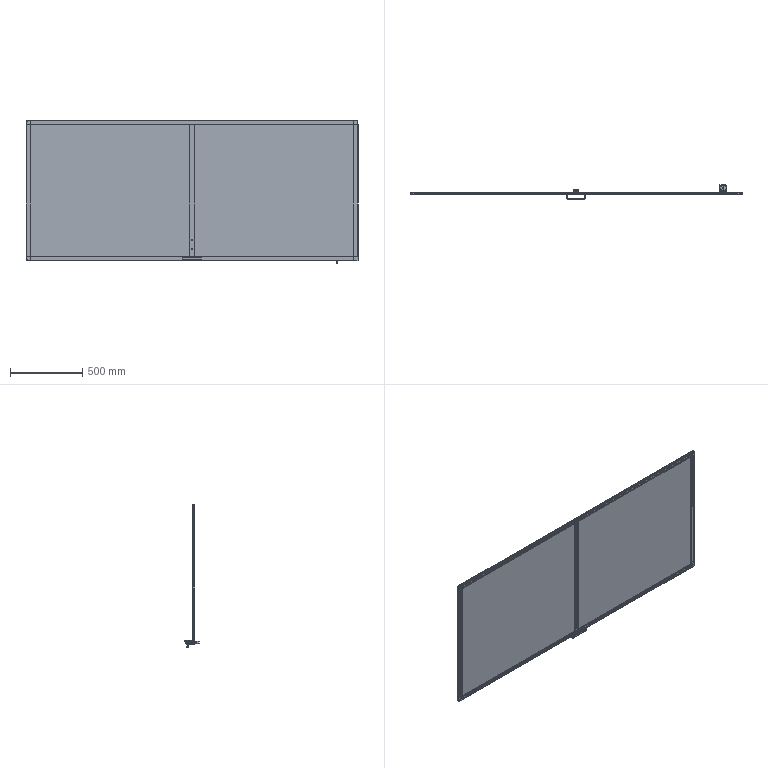Part | SolidWorks | features LocalLPattern 2, ReferencePattern 1 | 45 solids | 2388 faces | box 2296 x 97 x 991.55 mm | volume 12185495 mm3 | plane 1147 | cylinder 632 | cone 382 | spline 128 | torus 87 | sphere 12 | commonest cylinder face diameters 5 x103 1 x83 11 x52 4.5 x40 3.3 x28 6.5 x28